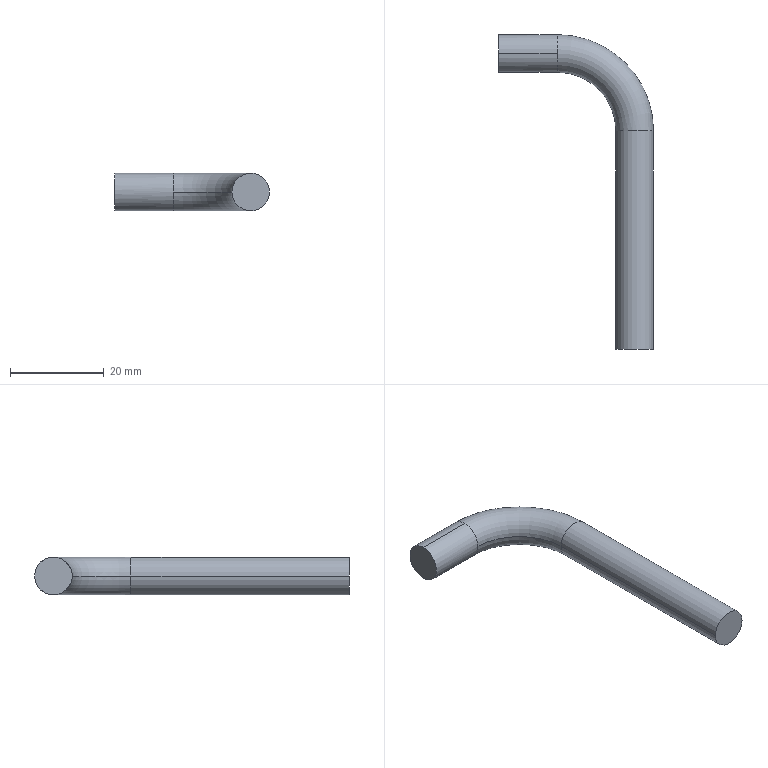Part | SolidWorks | features Sweep 1 | 1 solid | 8 faces | box 33 x 67 x 8 mm | volume 4268 mm3 | cylinder 4 | torus 2 | plane 2 | commonest cylinder face diameters 8 x4
STEP:
#1=CARTESIAN_POINT('',(12.5,0.,-4.));
#2=VERTEX_POINT('',#1);
#3=CARTESIAN_POINT('',(12.5,4.,0.));
#4=VERTEX_POINT('',#3);
#5=CARTESIAN_POINT('',(12.5,0.,0.));
#6=DIRECTION('',(1.,0.,0.));
#7=DIRECTION('',(0.,0.,-1.));
#8=AXIS2_PLACEMENT_3D('',#5,#6,#7);
#9=CIRCLE('',#8,4.);
#10=EDGE_CURVE('',#2,#4,#9,.T.);
#11=ORIENTED_EDGE('',*,*,#10,.T.);
#12=CARTESIAN_POINT('',(33.,-16.5,0.));
#13=VERTEX_POINT('',#12);
#14=CARTESIAN_POINT('',(12.5,-16.5,0.));
#15=DIRECTION('',(0.,0.,-1.));
#16=DIRECTION('',(-1.,0.,0.));
#17=AXIS2_PLACEMENT_3D('',#14,#15,#16);
#18=CIRCLE('',#17,20.5);
#19=EDGE_CURVE('',#4,#13,#18,.T.);
#20=ORIENTED_EDGE('',*,*,#19,.T.);
#21=CARTESIAN_POINT('',(25.,-16.5,0.));
#22=VERTEX_POINT('',#21);
#23=CARTESIAN_POINT('',(29.,-16.5,0.));
#24=DIRECTION('',(0.,-1.,0.));
#25=DIRECTION('',(0.,0.,-1.));
#26=AXIS2_PLACEMENT_3D('',#23,#24,#25);
#27=CIRCLE('',#26,4.);
#28=EDGE_CURVE('',#22,#13,#27,.T.);
#29=ORIENTED_EDGE('',*,*,#28,.F.);
#30=CARTESIAN_POINT('',(12.5,-4.,0.));
#31=VERTEX_POINT('',#30);
#32=CARTESIAN_POINT('',(12.5,-16.5,0.));
#33=DIRECTION('',(0.,0.,-1.));
#34=DIRECTION('',(-1.,0.,0.));
#35=AXIS2_PLACEMENT_3D('',#32,#33,#34);
#36=CIRCLE('',#35,12.5);
#37=EDGE_CURVE('',#31,#22,#36,.T.);
#38=ORIENTED_EDGE('',*,*,#37,.F.);
#39=CARTESIAN_POINT('',(12.5,0.,0.));
#40=DIRECTION('',(1.,0.,0.));
#41=DIRECTION('',(0.,0.,-1.));
#42=AXIS2_PLACEMENT_3D('',#39,#40,#41);
#43=CIRCLE('',#42,4.);
#44=EDGE_CURVE('',#31,#2,#43,.T.);
#45=ORIENTED_EDGE('',*,*,#44,.T.);
#46=EDGE_LOOP('',(#11,#20,#29,#38,#45));
#47=FACE_OUTER_BOUND('',#46,.T.);
#48=CARTESIAN_POINT('',(12.5,-16.5,0.));
#49=DIRECTION('',(0.,0.,-1.));
#50=DIRECTION('',(-1.,0.,0.));
#51=AXIS2_PLACEMENT_3D('',#48,#49,#50);
#52=TOROIDAL_SURFACE('',#51,16.5,4.);
#53=ADVANCED_FACE('',(#47),#52,.T.);
#54=ORIENTED_EDGE('',*,*,#10,.F.);
#55=CARTESIAN_POINT('',(0.,0.,-4.));
#56=VERTEX_POINT('',#55);
#57=CARTESIAN_POINT('',(12.5,0.,-4.));
#58=DIRECTION('',(-1.,0.,0.));
#59=VECTOR('',#58,1000.);
#60=LINE('',#57,#59);
#61=EDGE_CURVE('',#2,#56,#60,.T.);
#62=ORIENTED_EDGE('',*,*,#61,.T.);
#63=CARTESIAN_POINT('',(0.,0.,4.));
#64=VERTEX_POINT('',#63);
#65=CARTESIAN_POINT('',(0.,0.,0.));
#66=DIRECTION('',(1.,0.,0.));
#67=DIRECTION('',(0.,0.,-1.));
#68=AXIS2_PLACEMENT_3D('',#65,#66,#67);
#69=CIRCLE('',#68,4.);
#70=EDGE_CURVE('',#56,#64,#69,.T.);
#71=ORIENTED_EDGE('',*,*,#70,.T.);
#72=CARTESIAN_POINT('',(12.5,0.,4.));
#73=VERTEX_POINT('',#72);
#74=CARTESIAN_POINT('',(12.5,0.,4.));
#75=DIRECTION('',(-1.,0.,0.));
#76=VECTOR('',#75,1000.);
#77=LINE('',#74,#76);
#78=EDGE_CURVE('',#73,#64,#77,.T.);
#79=ORIENTED_EDGE('',*,*,#78,.F.);
#80=CARTESIAN_POINT('',(12.5,0.,0.));
#81=DIRECTION('',(1.,0.,0.));
#82=DIRECTION('',(0.,0.,-1.));
#83=AXIS2_PLACEMENT_3D('',#80,#81,#82);
#84=CIRCLE('',#83,4.);
#85=EDGE_CURVE('',#4,#73,#84,.T.);
#86=ORIENTED_EDGE('',*,*,#85,.F.);
#87=EDGE_LOOP('',(#54,#62,#71,#79,#86));
#88=FACE_OUTER_BOUND('',#87,.T.);
#89=CARTESIAN_POINT('',(12.5,0.,0.));
#90=DIRECTION('',(-1.,0.,0.));
#91=DIRECTION('',(0.,0.,1.));
#92=AXIS2_PLACEMENT_3D('',#89,#90,#91);
#93=CYLINDRICAL_SURFACE('',#92,4.);
#94=ADVANCED_FACE('',(#88),#93,.T.);
#95=CARTESIAN_POINT('',(29.,-16.5,0.));
#96=DIRECTION('',(0.,-1.,0.));
#97=DIRECTION('',(0.,0.,-1.));
#98=AXIS2_PLACEMENT_3D('',#95,#96,#97);
#99=CIRCLE('',#98,4.);
#100=EDGE_CURVE('',#13,#22,#99,.T.);
#101=ORIENTED_EDGE('',*,*,#100,.T.);
#102=CARTESIAN_POINT('',(25.,-63.,0.));
#103=VERTEX_POINT('',#102);
#104=CARTESIAN_POINT('',(25.,-16.5,0.));
#105=DIRECTION('',(0.,-1.,0.));
#106=VECTOR('',#105,1000.);
#107=LINE('',#104,#106);
#108=EDGE_CURVE('',#22,#103,#107,.T.);
#109=ORIENTED_EDGE('',*,*,#108,.T.);
#110=CARTESIAN_POINT('',(33.,-63.,0.));
#111=VERTEX_POINT('',#110);
#112=CARTESIAN_POINT('',(29.,-63.,0.));
#113=DIRECTION('',(0.,-1.,0.));
#114=DIRECTION('',(0.,0.,-1.));
#115=AXIS2_PLACEMENT_3D('',#112,#113,#114);
#116=CIRCLE('',#115,4.);
#117=EDGE_CURVE('',#111,#103,#116,.T.);
#118=ORIENTED_EDGE('',*,*,#117,.F.);
#119=CARTESIAN_POINT('',(33.,-16.5,0.));
#120=DIRECTION('',(0.,-1.,0.));
#121=VECTOR('',#120,1000.);
#122=LINE('',#119,#121);
#123=EDGE_CURVE('',#13,#111,#122,.T.);
#124=ORIENTED_EDGE('',*,*,#123,.F.);
#125=EDGE_LOOP('',(#101,#109,#118,#124));
#126=FACE_OUTER_BOUND('',#125,.T.);
#127=CARTESIAN_POINT('',(29.,-16.5,0.));
#128=DIRECTION('',(0.,-1.,0.));
#129=DIRECTION('',(1.,0.,0.));
#130=AXIS2_PLACEMENT_3D('',#127,#128,#129);
#131=CYLINDRICAL_SURFACE('',#130,4.);
#132=ADVANCED_FACE('',(#126),#131,.T.);
#133=ORIENTED_EDGE('',*,*,#108,.F.);
#134=ORIENTED_EDGE('',*,*,#28,.T.);
#135=ORIENTED_EDGE('',*,*,#123,.T.);
#136=CARTESIAN_POINT('',(29.,-63.,0.));
#137=DIRECTION('',(0.,-1.,0.));
#138=DIRECTION('',(0.,0.,-1.));
#139=AXIS2_PLACEMENT_3D('',#136,#137,#138);
#140=CIRCLE('',#139,4.);
#141=EDGE_CURVE('',#103,#111,#140,.T.);
#142=ORIENTED_EDGE('',*,*,#141,.F.);
#143=EDGE_LOOP('',(#133,#134,#135,#142));
#144=FACE_OUTER_BOUND('',#143,.T.);
#145=CARTESIAN_POINT('',(29.,-16.5,0.));
#146=DIRECTION('',(0.,-1.,0.));
#147=DIRECTION('',(1.,0.,0.));
#148=AXIS2_PLACEMENT_3D('',#145,#146,#147);
#149=CYLINDRICAL_SURFACE('',#148,4.);
#150=ADVANCED_FACE('',(#144),#149,.T.);
#151=ORIENTED_EDGE('',*,*,#19,.F.);
#152=ORIENTED_EDGE('',*,*,#85,.T.);
#153=CARTESIAN_POINT('',(12.5,0.,0.));
#154=DIRECTION('',(1.,0.,0.));
#155=DIRECTION('',(0.,0.,-1.));
#156=AXIS2_PLACEMENT_3D('',#153,#154,#155);
#157=CIRCLE('',#156,4.);
#158=EDGE_CURVE('',#73,#31,#157,.T.);
#159=ORIENTED_EDGE('',*,*,#158,.T.);
#160=ORIENTED_EDGE('',*,*,#37,.T.);
#161=ORIENTED_EDGE('',*,*,#100,.F.);
#162=EDGE_LOOP('',(#151,#152,#159,#160,#161));
#163=FACE_OUTER_BOUND('',#162,.T.);
#164=CARTESIAN_POINT('',(12.5,-16.5,0.));
#165=DIRECTION('',(0.,0.,-1.));
#166=DIRECTION('',(-1.,0.,0.));
#167=AXIS2_PLACEMENT_3D('',#164,#165,#166);
#168=TOROIDAL_SURFACE('',#167,16.5,4.);
#169=ADVANCED_FACE('',(#163),#168,.T.);
#170=ORIENTED_EDGE('',*,*,#61,.F.);
#171=ORIENTED_EDGE('',*,*,#44,.F.);
#172=ORIENTED_EDGE('',*,*,#158,.F.);
#173=ORIENTED_EDGE('',*,*,#78,.T.);
#174=CARTESIAN_POINT('',(0.,0.,0.));
#175=DIRECTION('',(1.,0.,0.));
#176=DIRECTION('',(0.,0.,-1.));
#177=AXIS2_PLACEMENT_3D('',#174,#175,#176);
#178=CIRCLE('',#177,4.);
#179=EDGE_CURVE('',#64,#56,#178,.T.);
#180=ORIENTED_EDGE('',*,*,#179,.T.);
#181=EDGE_LOOP('',(#170,#171,#172,#173,#180));
#182=FACE_OUTER_BOUND('',#181,.T.);
#183=CARTESIAN_POINT('',(12.5,0.,0.));
#184=DIRECTION('',(-1.,0.,0.));
#185=DIRECTION('',(0.,0.,1.));
#186=AXIS2_PLACEMENT_3D('',#183,#184,#185);
#187=CYLINDRICAL_SURFACE('',#186,4.);
#188=ADVANCED_FACE('',(#182),#187,.T.);
#189=ORIENTED_EDGE('',*,*,#117,.T.);
#190=ORIENTED_EDGE('',*,*,#141,.T.);
#191=EDGE_LOOP('',(#189,#190));
#192=FACE_OUTER_BOUND('',#191,.T.);
#193=CARTESIAN_POINT('',(29.,-63.,0.));
#194=DIRECTION('',(0.,-1.,0.));
#195=DIRECTION('',(0.,0.,-1.));
#196=AXIS2_PLACEMENT_3D('',#193,#194,#195);
#197=PLANE('',#196);
#198=ADVANCED_FACE('',(#192),#197,.T.);
#199=ORIENTED_EDGE('',*,*,#179,.F.);
#200=ORIENTED_EDGE('',*,*,#70,.F.);
#201=EDGE_LOOP('',(#199,#200));
#202=FACE_OUTER_BOUND('',#201,.T.);
#203=CARTESIAN_POINT('',(0.,0.,0.));
#204=DIRECTION('',(1.,0.,0.));
#205=DIRECTION('',(0.,0.,-1.));
#206=AXIS2_PLACEMENT_3D('',#203,#204,#205);
#207=PLANE('',#206);
#208=ADVANCED_FACE('',(#202),#207,.F.);
#209=CLOSED_SHELL('',(#53,#94,#132,#150,#169,#188,#198,#208));
#210=MANIFOLD_SOLID_BREP('',#209);
#211=CARTESIAN_POINT('',(0.,0.,0.));
#212=DIRECTION('',(0.,0.,1.));
#213=DIRECTION('',(1.,0.,0.));
#214=AXIS2_PLACEMENT_3D('',#211,#212,#213);
#215=(LENGTH_UNIT()NAMED_UNIT(*)SI_UNIT(.MILLI.,.METRE.));
#216=UNCERTAINTY_MEASURE_WITH_UNIT(LENGTH_MEASURE(0.00001),#215,'','');
#217=(NAMED_UNIT(*)PLANE_ANGLE_UNIT()SI_UNIT($,.RADIAN.));
#218=(NAMED_UNIT(*)SI_UNIT($,.STERADIAN.)SOLID_ANGLE_UNIT());
#219=(GEOMETRIC_REPRESENTATION_CONTEXT(3)GLOBAL_UNCERTAINTY_ASSIGNED_CONTEXT((#216))GLOBAL_UNIT_ASSIGNED_CONTEXT((#215,#217,#218))REPRESENTATION_CONTEXT('',''));
#220=ADVANCED_BREP_SHAPE_REPRESENTATION('',(#210,#214),#219);